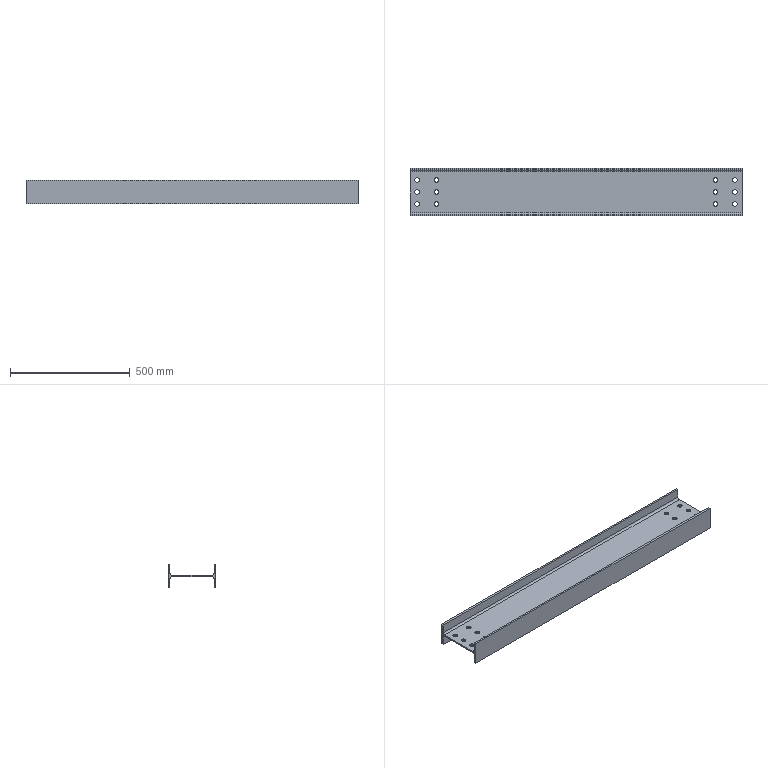Part | STEP file | 电柜通道主梁2主体_Default<As Machined> | 1 solid | 42 faces | box 1386 x 200 x 100 mm | volume 3677663 mm3 | cylinder 28 | plane 14 | commonest cylinder face diameters 19 x24 16 x4